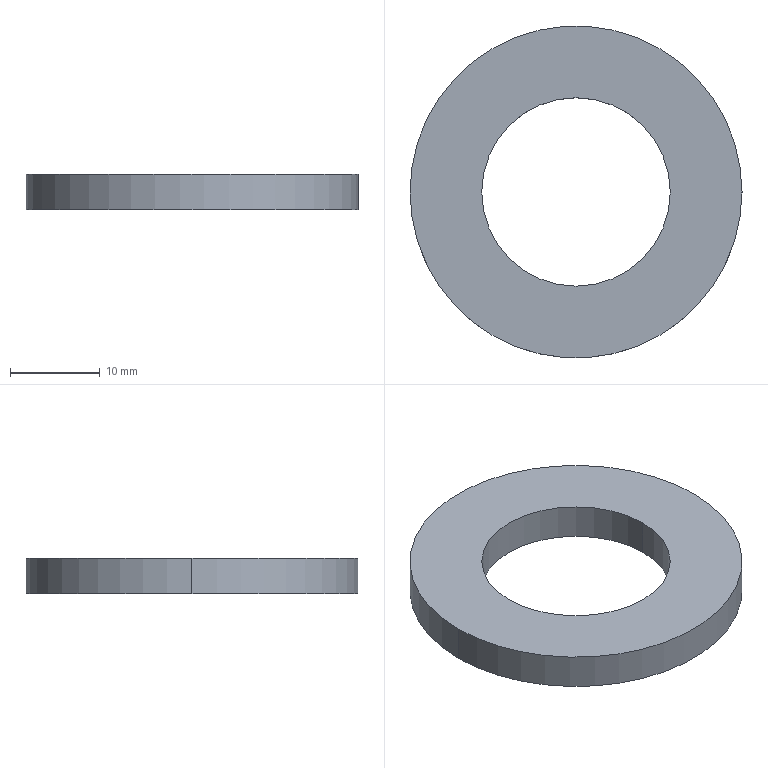Part | SolidWorks | features BaseBody 1 | 1 solid | 6 faces | box 37 x 37 x 4 mm | volume 2915 mm3 | cylinder 4 | plane 2 | commonest cylinder face diameters 21 x2 37 x2
STEP:
#1=CARTESIAN_POINT('',(18.5,0.,0.));
#2=VERTEX_POINT('',#1);
#3=CARTESIAN_POINT('',(-18.5,0.,0.));
#4=VERTEX_POINT('',#3);
#5=CARTESIAN_POINT('',(0.,0.,0.));
#6=DIRECTION('',(0.,0.,1.));
#7=DIRECTION('',(1.,0.,0.));
#8=AXIS2_PLACEMENT_3D('',#5,#6,#7);
#9=CIRCLE('',#8,18.5);
#10=EDGE_CURVE('',#2,#4,#9,.T.);
#11=ORIENTED_EDGE('',*,*,#10,.T.);
#12=CARTESIAN_POINT('',(-18.5,0.,4.));
#13=VERTEX_POINT('',#12);
#14=CARTESIAN_POINT('',(-18.5,0.,4.));
#15=DIRECTION('',(0.,0.,1.));
#16=VECTOR('',#15,1000.);
#17=LINE('',#14,#16);
#18=EDGE_CURVE('',#4,#13,#17,.T.);
#19=ORIENTED_EDGE('',*,*,#18,.T.);
#20=CARTESIAN_POINT('',(18.5,0.,4.));
#21=VERTEX_POINT('',#20);
#22=CARTESIAN_POINT('',(0.,0.,4.));
#23=DIRECTION('',(0.,0.,-1.));
#24=DIRECTION('',(1.,0.,0.));
#25=AXIS2_PLACEMENT_3D('',#22,#23,#24);
#26=CIRCLE('',#25,18.5);
#27=EDGE_CURVE('',#13,#21,#26,.T.);
#28=ORIENTED_EDGE('',*,*,#27,.T.);
#29=CARTESIAN_POINT('',(18.5,0.,4.));
#30=DIRECTION('',(0.,0.,1.));
#31=VECTOR('',#30,1000.);
#32=LINE('',#29,#31);
#33=EDGE_CURVE('',#2,#21,#32,.T.);
#34=ORIENTED_EDGE('',*,*,#33,.F.);
#35=EDGE_LOOP('',(#11,#19,#28,#34));
#36=FACE_OUTER_BOUND('',#35,.T.);
#37=CARTESIAN_POINT('',(0.,0.,4.));
#38=DIRECTION('',(0.,0.,1.));
#39=DIRECTION('',(1.,0.,0.));
#40=AXIS2_PLACEMENT_3D('',#37,#38,#39);
#41=CYLINDRICAL_SURFACE('',#40,18.5);
#42=ADVANCED_FACE('',(#36),#41,.T.);
#43=CARTESIAN_POINT('',(10.5,0.,0.));
#44=VERTEX_POINT('',#43);
#45=CARTESIAN_POINT('',(-10.5,0.,0.));
#46=VERTEX_POINT('',#45);
#47=CARTESIAN_POINT('',(0.,0.,0.));
#48=DIRECTION('',(0.,0.,-1.));
#49=DIRECTION('',(1.,0.,0.));
#50=AXIS2_PLACEMENT_3D('',#47,#48,#49);
#51=CIRCLE('',#50,10.5);
#52=EDGE_CURVE('',#44,#46,#51,.T.);
#53=ORIENTED_EDGE('',*,*,#52,.T.);
#54=CARTESIAN_POINT('',(-10.5,0.,4.));
#55=VERTEX_POINT('',#54);
#56=CARTESIAN_POINT('',(-10.5,0.,4.));
#57=DIRECTION('',(0.,0.,1.));
#58=VECTOR('',#57,1000.);
#59=LINE('',#56,#58);
#60=EDGE_CURVE('',#46,#55,#59,.T.);
#61=ORIENTED_EDGE('',*,*,#60,.T.);
#62=CARTESIAN_POINT('',(10.5,0.,4.));
#63=VERTEX_POINT('',#62);
#64=CARTESIAN_POINT('',(0.,0.,4.));
#65=DIRECTION('',(0.,0.,-1.));
#66=DIRECTION('',(1.,0.,0.));
#67=AXIS2_PLACEMENT_3D('',#64,#65,#66);
#68=CIRCLE('',#67,10.5);
#69=EDGE_CURVE('',#63,#55,#68,.T.);
#70=ORIENTED_EDGE('',*,*,#69,.F.);
#71=CARTESIAN_POINT('',(10.5,0.,4.));
#72=DIRECTION('',(0.,0.,1.));
#73=VECTOR('',#72,1000.);
#74=LINE('',#71,#73);
#75=EDGE_CURVE('',#44,#63,#74,.T.);
#76=ORIENTED_EDGE('',*,*,#75,.F.);
#77=EDGE_LOOP('',(#53,#61,#70,#76));
#78=FACE_OUTER_BOUND('',#77,.T.);
#79=CARTESIAN_POINT('',(0.,0.,4.));
#80=DIRECTION('',(0.,0.,1.));
#81=DIRECTION('',(1.,0.,0.));
#82=AXIS2_PLACEMENT_3D('',#79,#80,#81);
#83=CYLINDRICAL_SURFACE('',#82,10.5);
#84=ADVANCED_FACE('',(#78),#83,.F.);
#85=ORIENTED_EDGE('',*,*,#10,.F.);
#86=CARTESIAN_POINT('',(0.,0.,0.));
#87=DIRECTION('',(0.,0.,1.));
#88=DIRECTION('',(1.,0.,0.));
#89=AXIS2_PLACEMENT_3D('',#86,#87,#88);
#90=CIRCLE('',#89,18.5);
#91=EDGE_CURVE('',#4,#2,#90,.T.);
#92=ORIENTED_EDGE('',*,*,#91,.F.);
#93=EDGE_LOOP('',(#85,#92));
#94=FACE_OUTER_BOUND('',#93,.T.);
#95=ORIENTED_EDGE('',*,*,#52,.F.);
#96=CARTESIAN_POINT('',(0.,0.,0.));
#97=DIRECTION('',(0.,0.,-1.));
#98=DIRECTION('',(1.,0.,0.));
#99=AXIS2_PLACEMENT_3D('',#96,#97,#98);
#100=CIRCLE('',#99,10.5);
#101=EDGE_CURVE('',#46,#44,#100,.T.);
#102=ORIENTED_EDGE('',*,*,#101,.F.);
#103=EDGE_LOOP('',(#95,#102));
#104=FACE_BOUND('',#103,.T.);
#105=CARTESIAN_POINT('',(0.,0.,0.));
#106=DIRECTION('',(0.,0.,1.));
#107=DIRECTION('',(1.,0.,0.));
#108=AXIS2_PLACEMENT_3D('',#105,#106,#107);
#109=PLANE('',#108);
#110=ADVANCED_FACE('',(#94,#104),#109,.F.);
#111=ORIENTED_EDGE('',*,*,#18,.F.);
#112=ORIENTED_EDGE('',*,*,#91,.T.);
#113=ORIENTED_EDGE('',*,*,#33,.T.);
#114=CARTESIAN_POINT('',(0.,0.,4.));
#115=DIRECTION('',(0.,0.,-1.));
#116=DIRECTION('',(1.,0.,0.));
#117=AXIS2_PLACEMENT_3D('',#114,#115,#116);
#118=CIRCLE('',#117,18.5);
#119=EDGE_CURVE('',#21,#13,#118,.T.);
#120=ORIENTED_EDGE('',*,*,#119,.T.);
#121=EDGE_LOOP('',(#111,#112,#113,#120));
#122=FACE_OUTER_BOUND('',#121,.T.);
#123=CARTESIAN_POINT('',(0.,0.,4.));
#124=DIRECTION('',(0.,0.,1.));
#125=DIRECTION('',(1.,0.,0.));
#126=AXIS2_PLACEMENT_3D('',#123,#124,#125);
#127=CYLINDRICAL_SURFACE('',#126,18.5);
#128=ADVANCED_FACE('',(#122),#127,.T.);
#129=ORIENTED_EDGE('',*,*,#60,.F.);
#130=ORIENTED_EDGE('',*,*,#101,.T.);
#131=ORIENTED_EDGE('',*,*,#75,.T.);
#132=CARTESIAN_POINT('',(0.,0.,4.));
#133=DIRECTION('',(0.,0.,-1.));
#134=DIRECTION('',(1.,0.,0.));
#135=AXIS2_PLACEMENT_3D('',#132,#133,#134);
#136=CIRCLE('',#135,10.5);
#137=EDGE_CURVE('',#55,#63,#136,.T.);
#138=ORIENTED_EDGE('',*,*,#137,.F.);
#139=EDGE_LOOP('',(#129,#130,#131,#138));
#140=FACE_OUTER_BOUND('',#139,.T.);
#141=CARTESIAN_POINT('',(0.,0.,4.));
#142=DIRECTION('',(0.,0.,1.));
#143=DIRECTION('',(1.,0.,0.));
#144=AXIS2_PLACEMENT_3D('',#141,#142,#143);
#145=CYLINDRICAL_SURFACE('',#144,10.5);
#146=ADVANCED_FACE('',(#140),#145,.F.);
#147=ORIENTED_EDGE('',*,*,#119,.F.);
#148=ORIENTED_EDGE('',*,*,#27,.F.);
#149=EDGE_LOOP('',(#147,#148));
#150=FACE_OUTER_BOUND('',#149,.T.);
#151=ORIENTED_EDGE('',*,*,#69,.T.);
#152=ORIENTED_EDGE('',*,*,#137,.T.);
#153=EDGE_LOOP('',(#151,#152));
#154=FACE_BOUND('',#153,.T.);
#155=CARTESIAN_POINT('',(0.,0.,4.));
#156=DIRECTION('',(0.,0.,1.));
#157=DIRECTION('',(1.,0.,0.));
#158=AXIS2_PLACEMENT_3D('',#155,#156,#157);
#159=PLANE('',#158);
#160=ADVANCED_FACE('',(#150,#154),#159,.T.);
#161=CLOSED_SHELL('',(#42,#84,#110,#128,#146,#160));
#162=MANIFOLD_SOLID_BREP('',#161);
#163=CARTESIAN_POINT('',(0.,0.,0.));
#164=DIRECTION('',(0.,0.,1.));
#165=DIRECTION('',(1.,0.,0.));
#166=AXIS2_PLACEMENT_3D('',#163,#164,#165);
#167=(LENGTH_UNIT()NAMED_UNIT(*)SI_UNIT(.MILLI.,.METRE.));
#168=UNCERTAINTY_MEASURE_WITH_UNIT(LENGTH_MEASURE(0.00001),#167,'','');
#169=(NAMED_UNIT(*)PLANE_ANGLE_UNIT()SI_UNIT($,.RADIAN.));
#170=(NAMED_UNIT(*)SI_UNIT($,.STERADIAN.)SOLID_ANGLE_UNIT());
#171=(GEOMETRIC_REPRESENTATION_CONTEXT(3)GLOBAL_UNCERTAINTY_ASSIGNED_CONTEXT((#168))GLOBAL_UNIT_ASSIGNED_CONTEXT((#167,#169,#170))REPRESENTATION_CONTEXT('',''));
#172=ADVANCED_BREP_SHAPE_REPRESENTATION('',(#162,#166),#171);